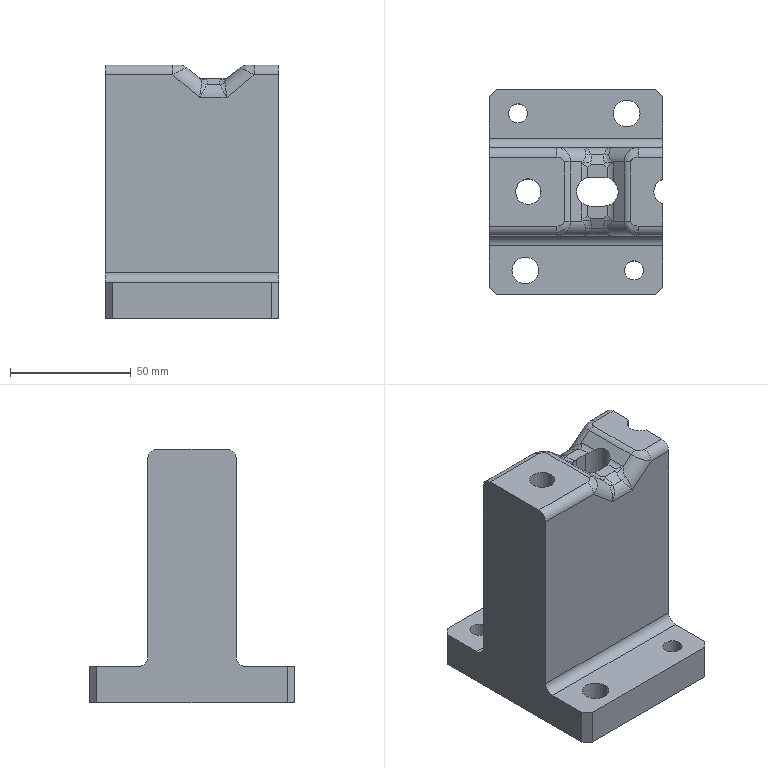Part | STEP file | 1_id62_x_t | 1 solid | 84 faces | box 72 x 85 x 105 mm | volume 283891 mm3 | cylinder 36 | plane 32 | spline 16 | commonest cylinder face diameters 8 x12 12 x8 6 x4 7.938 x4 11 x4 10.524 x2